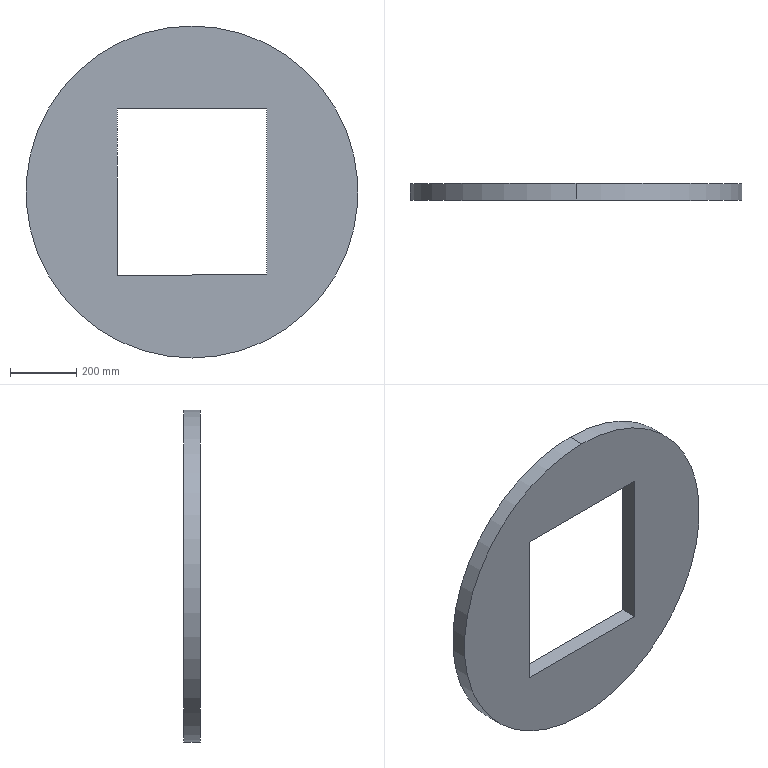Part | SolidWorks | features Cut 1, Extrusion 1 | 1 solid | 8 faces | box 1000 x 50 x 1000 mm | volume 28019908 mm3 | plane 6 | cylinder 2 | commonest cylinder face diameters 1000 x2
STEP:
#1=CARTESIAN_POINT('',(0.,50.,500.));
#2=VERTEX_POINT('',#1);
#3=CARTESIAN_POINT('',(0.,50.,-500.));
#4=VERTEX_POINT('',#3);
#5=CARTESIAN_POINT('',(0.,50.,0.));
#6=DIRECTION('',(0.,1.,0.));
#7=DIRECTION('',(0.,0.,1.));
#8=AXIS2_PLACEMENT_3D('',#5,#6,#7);
#9=CIRCLE('',#8,500.);
#10=EDGE_CURVE('',#2,#4,#9,.T.);
#11=ORIENTED_EDGE('',*,*,#10,.F.);
#12=CARTESIAN_POINT('',(0.,0.,500.));
#13=VERTEX_POINT('',#12);
#14=CARTESIAN_POINT('',(0.,50.,500.));
#15=DIRECTION('',(0.,-1.,0.));
#16=VECTOR('',#15,1000.);
#17=LINE('',#14,#16);
#18=EDGE_CURVE('',#2,#13,#17,.T.);
#19=ORIENTED_EDGE('',*,*,#18,.T.);
#20=CARTESIAN_POINT('',(0.,0.,-500.));
#21=VERTEX_POINT('',#20);
#22=CARTESIAN_POINT('',(0.,0.,0.));
#23=DIRECTION('',(0.,1.,0.));
#24=DIRECTION('',(0.,0.,1.));
#25=AXIS2_PLACEMENT_3D('',#22,#23,#24);
#26=CIRCLE('',#25,500.);
#27=EDGE_CURVE('',#13,#21,#26,.T.);
#28=ORIENTED_EDGE('',*,*,#27,.T.);
#29=CARTESIAN_POINT('',(0.,50.,-500.));
#30=DIRECTION('',(0.,-1.,0.));
#31=VECTOR('',#30,1000.);
#32=LINE('',#29,#31);
#33=EDGE_CURVE('',#4,#21,#32,.T.);
#34=ORIENTED_EDGE('',*,*,#33,.F.);
#35=EDGE_LOOP('',(#11,#19,#28,#34));
#36=FACE_OUTER_BOUND('',#35,.T.);
#37=CARTESIAN_POINT('',(0.,50.,0.));
#38=DIRECTION('',(0.,-1.,0.));
#39=DIRECTION('',(0.,0.,-1.));
#40=AXIS2_PLACEMENT_3D('',#37,#38,#39);
#41=CYLINDRICAL_SURFACE('',#40,500.);
#42=ADVANCED_FACE('',(#36),#41,.T.);
#43=ORIENTED_EDGE('',*,*,#18,.F.);
#44=CARTESIAN_POINT('',(0.,50.,0.));
#45=DIRECTION('',(0.,1.,0.));
#46=DIRECTION('',(0.,0.,1.));
#47=AXIS2_PLACEMENT_3D('',#44,#45,#46);
#48=CIRCLE('',#47,500.);
#49=EDGE_CURVE('',#4,#2,#48,.T.);
#50=ORIENTED_EDGE('',*,*,#49,.F.);
#51=ORIENTED_EDGE('',*,*,#33,.T.);
#52=CARTESIAN_POINT('',(0.,0.,0.));
#53=DIRECTION('',(0.,1.,0.));
#54=DIRECTION('',(0.,0.,1.));
#55=AXIS2_PLACEMENT_3D('',#52,#53,#54);
#56=CIRCLE('',#55,500.);
#57=EDGE_CURVE('',#21,#13,#56,.T.);
#58=ORIENTED_EDGE('',*,*,#57,.T.);
#59=EDGE_LOOP('',(#43,#50,#51,#58));
#60=FACE_OUTER_BOUND('',#59,.T.);
#61=CARTESIAN_POINT('',(0.,50.,0.));
#62=DIRECTION('',(0.,-1.,0.));
#63=DIRECTION('',(0.,0.,-1.));
#64=AXIS2_PLACEMENT_3D('',#61,#62,#63);
#65=CYLINDRICAL_SURFACE('',#64,500.);
#66=ADVANCED_FACE('',(#60),#65,.T.);
#67=CARTESIAN_POINT('',(225.,50.,250.));
#68=VERTEX_POINT('',#67);
#69=CARTESIAN_POINT('',(225.,50.,-250.));
#70=VERTEX_POINT('',#69);
#71=CARTESIAN_POINT('',(225.,50.,0.));
#72=DIRECTION('',(0.,0.,-1.));
#73=VECTOR('',#72,1000.);
#74=LINE('',#71,#73);
#75=EDGE_CURVE('',#68,#70,#74,.T.);
#76=ORIENTED_EDGE('',*,*,#75,.F.);
#77=CARTESIAN_POINT('',(-225.,50.,250.));
#78=VERTEX_POINT('',#77);
#79=CARTESIAN_POINT('',(0.,50.,250.));
#80=DIRECTION('',(1.,0.,0.));
#81=VECTOR('',#80,1000.);
#82=LINE('',#79,#81);
#83=EDGE_CURVE('',#78,#68,#82,.T.);
#84=ORIENTED_EDGE('',*,*,#83,.F.);
#85=CARTESIAN_POINT('',(-225.,50.,-250.));
#86=VERTEX_POINT('',#85);
#87=CARTESIAN_POINT('',(-225.,50.,0.));
#88=DIRECTION('',(0.,0.,1.));
#89=VECTOR('',#88,1000.);
#90=LINE('',#87,#89);
#91=EDGE_CURVE('',#86,#78,#90,.T.);
#92=ORIENTED_EDGE('',*,*,#91,.F.);
#93=CARTESIAN_POINT('',(0.,50.,-250.));
#94=DIRECTION('',(-1.,0.,0.));
#95=VECTOR('',#94,1000.);
#96=LINE('',#93,#95);
#97=EDGE_CURVE('',#70,#86,#96,.T.);
#98=ORIENTED_EDGE('',*,*,#97,.F.);
#99=EDGE_LOOP('',(#76,#84,#92,#98));
#100=FACE_BOUND('',#99,.T.);
#101=ORIENTED_EDGE('',*,*,#49,.T.);
#102=ORIENTED_EDGE('',*,*,#10,.T.);
#103=EDGE_LOOP('',(#101,#102));
#104=FACE_OUTER_BOUND('',#103,.T.);
#105=CARTESIAN_POINT('',(0.,50.,0.));
#106=DIRECTION('',(0.,1.,0.));
#107=DIRECTION('',(0.,0.,1.));
#108=AXIS2_PLACEMENT_3D('',#105,#106,#107);
#109=PLANE('',#108);
#110=ADVANCED_FACE('',(#100,#104),#109,.T.);
#111=CARTESIAN_POINT('',(-225.,0.,250.));
#112=VERTEX_POINT('',#111);
#113=CARTESIAN_POINT('',(225.,0.,250.));
#114=VERTEX_POINT('',#113);
#115=CARTESIAN_POINT('',(-225.,0.,250.));
#116=DIRECTION('',(1.,0.,0.));
#117=VECTOR('',#116,1000.);
#118=LINE('',#115,#117);
#119=EDGE_CURVE('',#112,#114,#118,.T.);
#120=ORIENTED_EDGE('',*,*,#119,.T.);
#121=CARTESIAN_POINT('',(225.,0.,-250.));
#122=VERTEX_POINT('',#121);
#123=CARTESIAN_POINT('',(225.,0.,-250.));
#124=DIRECTION('',(0.,0.,-1.));
#125=VECTOR('',#124,1000.);
#126=LINE('',#123,#125);
#127=EDGE_CURVE('',#114,#122,#126,.T.);
#128=ORIENTED_EDGE('',*,*,#127,.T.);
#129=CARTESIAN_POINT('',(-225.,0.,-250.));
#130=VERTEX_POINT('',#129);
#131=CARTESIAN_POINT('',(-225.,0.,-250.));
#132=DIRECTION('',(-1.,0.,0.));
#133=VECTOR('',#132,1000.);
#134=LINE('',#131,#133);
#135=EDGE_CURVE('',#122,#130,#134,.T.);
#136=ORIENTED_EDGE('',*,*,#135,.T.);
#137=CARTESIAN_POINT('',(-225.,0.,-250.));
#138=DIRECTION('',(0.,0.,1.));
#139=VECTOR('',#138,1000.);
#140=LINE('',#137,#139);
#141=EDGE_CURVE('',#130,#112,#140,.T.);
#142=ORIENTED_EDGE('',*,*,#141,.T.);
#143=EDGE_LOOP('',(#120,#128,#136,#142));
#144=FACE_BOUND('',#143,.T.);
#145=ORIENTED_EDGE('',*,*,#57,.F.);
#146=ORIENTED_EDGE('',*,*,#27,.F.);
#147=EDGE_LOOP('',(#145,#146));
#148=FACE_OUTER_BOUND('',#147,.T.);
#149=CARTESIAN_POINT('',(0.,0.,0.));
#150=DIRECTION('',(0.,1.,0.));
#151=DIRECTION('',(0.,0.,1.));
#152=AXIS2_PLACEMENT_3D('',#149,#150,#151);
#153=PLANE('',#152);
#154=ADVANCED_FACE('',(#144,#148),#153,.F.);
#155=ORIENTED_EDGE('',*,*,#75,.T.);
#156=CARTESIAN_POINT('',(225.,0.,-250.));
#157=DIRECTION('',(0.,1.,0.));
#158=VECTOR('',#157,1000.);
#159=LINE('',#156,#158);
#160=EDGE_CURVE('',#122,#70,#159,.T.);
#161=ORIENTED_EDGE('',*,*,#160,.F.);
#162=ORIENTED_EDGE('',*,*,#127,.F.);
#163=CARTESIAN_POINT('',(225.,0.,250.));
#164=DIRECTION('',(0.,1.,0.));
#165=VECTOR('',#164,1000.);
#166=LINE('',#163,#165);
#167=EDGE_CURVE('',#114,#68,#166,.T.);
#168=ORIENTED_EDGE('',*,*,#167,.T.);
#169=EDGE_LOOP('',(#155,#161,#162,#168));
#170=FACE_OUTER_BOUND('',#169,.T.);
#171=CARTESIAN_POINT('',(225.,0.,-250.));
#172=DIRECTION('',(1.,0.,0.));
#173=DIRECTION('',(0.,0.,-1.));
#174=AXIS2_PLACEMENT_3D('',#171,#172,#173);
#175=PLANE('',#174);
#176=ADVANCED_FACE('',(#170),#175,.F.);
#177=ORIENTED_EDGE('',*,*,#83,.T.);
#178=ORIENTED_EDGE('',*,*,#167,.F.);
#179=ORIENTED_EDGE('',*,*,#119,.F.);
#180=CARTESIAN_POINT('',(-225.,0.,250.));
#181=DIRECTION('',(0.,1.,0.));
#182=VECTOR('',#181,1000.);
#183=LINE('',#180,#182);
#184=EDGE_CURVE('',#112,#78,#183,.T.);
#185=ORIENTED_EDGE('',*,*,#184,.T.);
#186=EDGE_LOOP('',(#177,#178,#179,#185));
#187=FACE_OUTER_BOUND('',#186,.T.);
#188=CARTESIAN_POINT('',(-225.,0.,250.));
#189=DIRECTION('',(0.,0.,1.));
#190=DIRECTION('',(1.,0.,0.));
#191=AXIS2_PLACEMENT_3D('',#188,#189,#190);
#192=PLANE('',#191);
#193=ADVANCED_FACE('',(#187),#192,.F.);
#194=ORIENTED_EDGE('',*,*,#91,.T.);
#195=ORIENTED_EDGE('',*,*,#184,.F.);
#196=ORIENTED_EDGE('',*,*,#141,.F.);
#197=CARTESIAN_POINT('',(-225.,0.,-250.));
#198=DIRECTION('',(0.,1.,0.));
#199=VECTOR('',#198,1000.);
#200=LINE('',#197,#199);
#201=EDGE_CURVE('',#130,#86,#200,.T.);
#202=ORIENTED_EDGE('',*,*,#201,.T.);
#203=EDGE_LOOP('',(#194,#195,#196,#202));
#204=FACE_OUTER_BOUND('',#203,.T.);
#205=CARTESIAN_POINT('',(-225.,0.,-250.));
#206=DIRECTION('',(-1.,0.,0.));
#207=DIRECTION('',(0.,0.,1.));
#208=AXIS2_PLACEMENT_3D('',#205,#206,#207);
#209=PLANE('',#208);
#210=ADVANCED_FACE('',(#204),#209,.F.);
#211=ORIENTED_EDGE('',*,*,#97,.T.);
#212=ORIENTED_EDGE('',*,*,#201,.F.);
#213=ORIENTED_EDGE('',*,*,#135,.F.);
#214=ORIENTED_EDGE('',*,*,#160,.T.);
#215=EDGE_LOOP('',(#211,#212,#213,#214));
#216=FACE_OUTER_BOUND('',#215,.T.);
#217=CARTESIAN_POINT('',(-225.,0.,-250.));
#218=DIRECTION('',(0.,0.,-1.));
#219=DIRECTION('',(-1.,0.,0.));
#220=AXIS2_PLACEMENT_3D('',#217,#218,#219);
#221=PLANE('',#220);
#222=ADVANCED_FACE('',(#216),#221,.F.);
#223=CLOSED_SHELL('',(#42,#66,#110,#154,#176,#193,#210,#222));
#224=MANIFOLD_SOLID_BREP('',#223);
#225=CARTESIAN_POINT('',(0.,0.,0.));
#226=DIRECTION('',(0.,0.,1.));
#227=DIRECTION('',(1.,0.,0.));
#228=AXIS2_PLACEMENT_3D('',#225,#226,#227);
#229=(LENGTH_UNIT()NAMED_UNIT(*)SI_UNIT(.MILLI.,.METRE.));
#230=UNCERTAINTY_MEASURE_WITH_UNIT(LENGTH_MEASURE(0.00001),#229,'','');
#231=(NAMED_UNIT(*)PLANE_ANGLE_UNIT()SI_UNIT($,.RADIAN.));
#232=(NAMED_UNIT(*)SI_UNIT($,.STERADIAN.)SOLID_ANGLE_UNIT());
#233=(GEOMETRIC_REPRESENTATION_CONTEXT(3)GLOBAL_UNCERTAINTY_ASSIGNED_CONTEXT((#230))GLOBAL_UNIT_ASSIGNED_CONTEXT((#229,#231,#232))REPRESENTATION_CONTEXT('',''));
#234=ADVANCED_BREP_SHAPE_REPRESENTATION('',(#224,#228),#233);